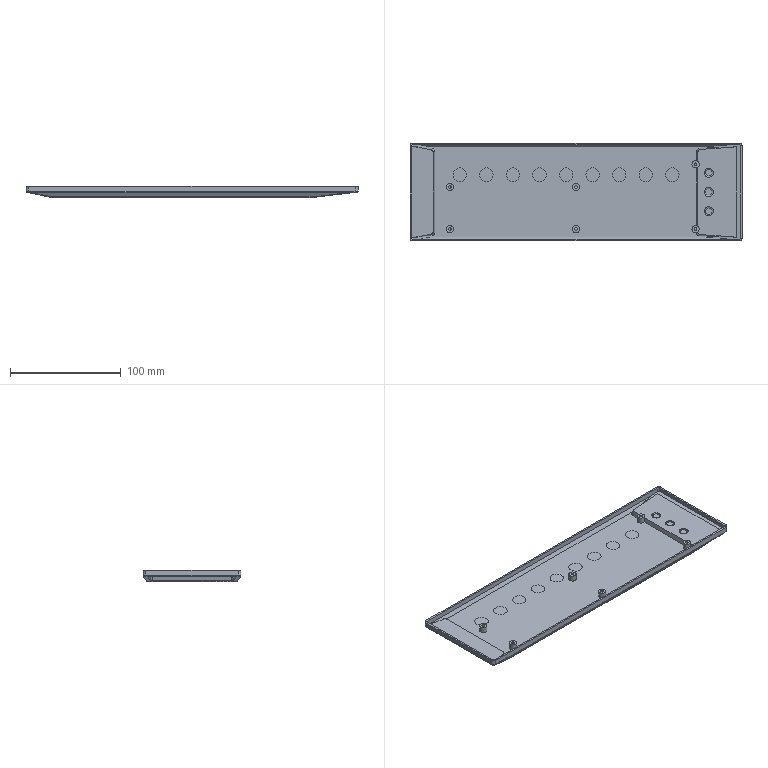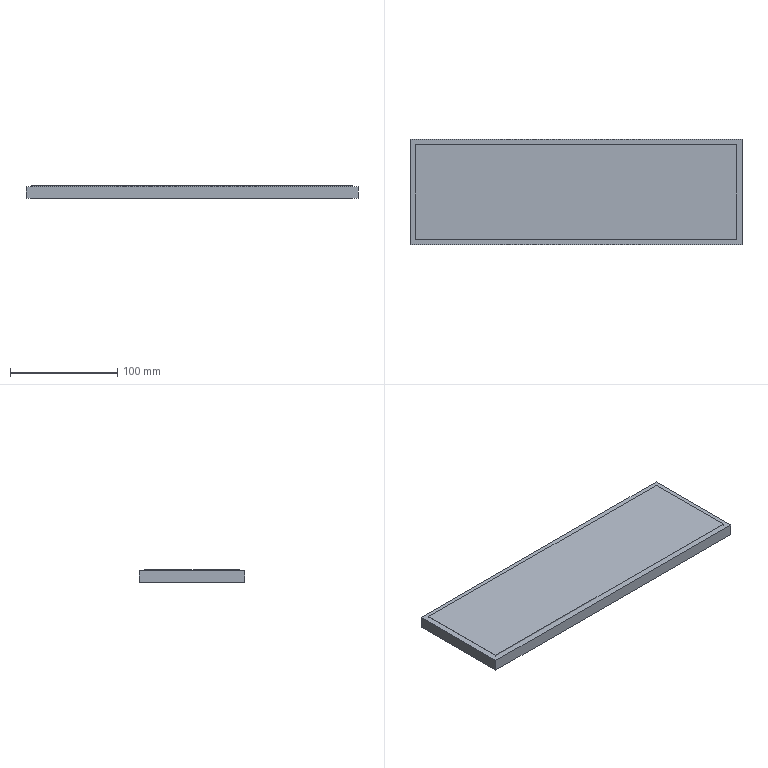CAM job | NX | 3-axis milling, drilling | part box 300 x 88.5 x 10 mm | stock box 310 x 98.5 x 12 mm
Tools:
number,name,description,diameter,corner_radius,flute_length,length,flutes
1,D63,Milling Tool-5 Parameters,63.0,0.0,50.0,75.0,2
8,D8,Milling Tool-5 Parameters,8.0,0.0,50.0,75.0,2
4,D4,Milling Tool-5 Parameters,4.0,0.0,50.0,75.0,2
2,D2,Milling Tool-5 Parameters,2.0,0.0,50.0,75.0,2
11,D1.5,Milling Tool-5 Parameters,1.5,0.0,50.0,75.0,2
5,D2R0.5,Milling Tool-5 Parameters,2.0,0.5,50.0,75.0,2
7,D4A45,Milling Tool-5 Parameters,4.0,0.0,50.0,75.0,2
12,2.5ZT,Drilling Tool,2.5,0.0,35.0,50.0,2
9,D3R0.5,Milling Tool-5 Parameters,3.0,0.5,50.0,75.0,2
Operations:
program,operation,operation_type,tool,method,geometry_group,spindle_rpm,surface_speed,feed_per_tooth,feed_cut,feed_plunge,cut_length_mm,path_length_mm,cut_time_min,machine_time_min
1,FLOOR_WALL,VolumeBased25DMillingOperation,D63,METHOD,A,6500.0,1286.0,0.0962,1250.0,100.0,1204.297,1258.297,0.9634,0.9688
1,ADAPTIVE_MILLING,CavityMilling,D8,METHOD,A,9500.0,238.0,0.1579,3000.0,1000.0,5010.781,5084.781,1.672,1.68
1,ZLEVEL_PROFILE,ZLevelMilling,D8,METHOD,A,9500.0,238.0,0.0658,1250.0,100.0,805.162,882.162,0.6441,0.6518
1,CAVITY_MILL,CavityMilling,D8,METHOD,A,9500.0,238.0,0.1579,3000.0,1000.0,52990.021,55506.314,18.731,18.982
1,CAVITY_MILL_COPY,CavityMilling,D4,METHOD,A,9500.0,119.0,0.0868,1650.0,1000.0,4445.12,7837.169,3.484,3.823
1,FLOOR_WALL_1,VolumeBased25DMillingOperation,D4,METHOD,A,9500.0,119.0,0.0658,1250.0,100.0,12889.863,15791.57,10.312,10.602
1,CAVITY_MILL_COPY_COPY,CavityMilling,D2,METHOD,A,9500.0,59.0,0.0579,1100.0,1000.0,3155.138,5673.696,2.91,3.162
1,CAVITY_MILL_COPY_COPY_COPY_1,CavityMilling,D2,METHOD,A,9500.0,59.0,0.0526,1000.0,1000.0,3043.425,3109.213,3.043,3.05
1,ZLEVEL_PROFILE_1,ZLevelMilling,D2,METHOD,A,9500.0,59.0,0.0658,1250.0,100.0,325.681,1187.015,0.2605,0.3467
1,ZLEVEL_PROFILE_1_COPY,ZLevelMilling,D2,METHOD,A,9500.0,59.0,0.0658,1250.0,100.0,52.201,296.07,0.0418,0.0661
1,FIXED_CONTOUR,SurfaceContour,D2R0.5,METHOD,A,9500.0,59.0,0.1316,2500.0,1000.0,49633.025,51178.987,19.933,20.088
1,CAVITY_MILL_COPY_COPY_COPY,CavityMilling,D1.5,METHOD,A,9500.0,29.0,0.0447,850.0,1000.0,5283.086,9349.664,6.065,6.471
1,DRILLING,Operation,D4A45,METHOD,A,5000.0,62.0,0.025,250.0,0.0,27.6,492.094,0.1104,0.1568
1,DRILLING_COPY,Operation,2.5ZT,METHOD,A,2000.0,15.0,0.025,100.0,0.0,51.0,538.894,0.51,0.5588
1,PLANAR_MILL,PlanarMilling,D4A45,METHOD,A,9500.0,119.0,0.0658,1250.0,100.0,1546.18,1751.146,1.237,1.257
2,FLOOR_WALL_COPY,VolumeBased25DMillingOperation,D63,METHOD,B,6500.0,1286.0,0.0962,1250.0,100.0,4673.188,6018.186,3.739,3.873
2,CAVITY_MILL_COPY_1,CavityMilling,D8,METHOD,B,9500.0,238.0,0.1579,3000.0,1000.0,28609.589,30646.562,9.69,9.894
2,CAVITY_MILL_COPY_COPY_1,CavityMilling,D4,METHOD,B,9500.0,119.0,0.0868,1650.0,1000.0,1048.141,3972.522,0.8132,1.106
2,FLOOR_WALL_1_COPY,VolumeBased25DMillingOperation,D4,METHOD,B,9500.0,119.0,0.0658,1250.0,100.0,13168.445,14086.038,10.535,10.627
2,CAVITY_MILL_COPY_COPY_COPY_2,CavityMilling,D2,METHOD,B,9500.0,59.0,0.0579,1100.0,1000.0,2918.366,5216.662,2.662,2.892
2,FIXED_CONTOUR_COPY,SurfaceContour,D3R0.5,METHOD,B,9500.0,89.0,0.1316,2500.0,1000.0,116127.682,118369.799,46.524,46.748
2,PLANAR_MILL_COPY,PlanarMilling,D4A45,METHOD,B,9500.0,119.0,0.0658,1250.0,100.0,337.075,1078.574,0.2697,0.3438
3,FIXED_CONTOUR_COPY_COPY,SurfaceContour,D3R0.5,METHOD,B,9500.0,89.0,0.1316,2500.0,1000.0,22695.434,23046.483,9.145,9.18